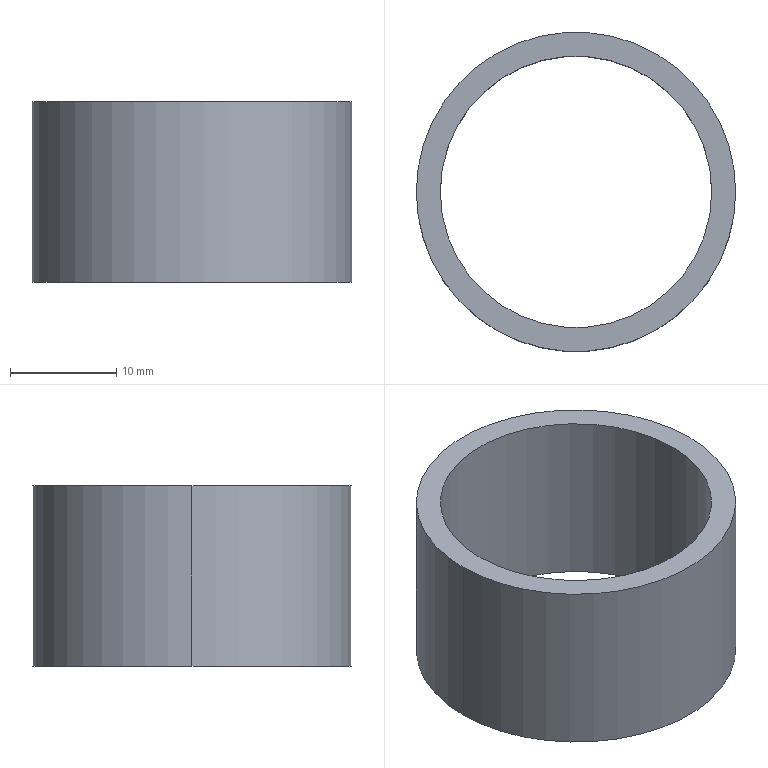Part | SolidWorks | features Extrusion 1 | 1 solid | 6 faces | box 30 x 30 x 17 mm | volume 3335 mm3 | cylinder 4 | plane 2 | commonest cylinder face diameters 25.5 x2 30 x2
STEP:
#1=CARTESIAN_POINT('',(-12.75,0.,17.));
#2=VERTEX_POINT('',#1);
#3=CARTESIAN_POINT('',(12.75,0.,17.));
#4=VERTEX_POINT('',#3);
#5=CARTESIAN_POINT('',(0.,0.,17.));
#6=DIRECTION('',(0.,0.,1.));
#7=DIRECTION('',(1.,0.,0.));
#8=AXIS2_PLACEMENT_3D('',#5,#6,#7);
#9=CIRCLE('',#8,12.75);
#10=EDGE_CURVE('',#2,#4,#9,.T.);
#11=ORIENTED_EDGE('',*,*,#10,.T.);
#12=CARTESIAN_POINT('',(12.75,0.,0.));
#13=VERTEX_POINT('',#12);
#14=CARTESIAN_POINT('',(12.75,0.,17.));
#15=DIRECTION('',(0.,0.,-1.));
#16=VECTOR('',#15,1000.);
#17=LINE('',#14,#16);
#18=EDGE_CURVE('',#4,#13,#17,.T.);
#19=ORIENTED_EDGE('',*,*,#18,.T.);
#20=CARTESIAN_POINT('',(-12.75,0.,0.));
#21=VERTEX_POINT('',#20);
#22=CARTESIAN_POINT('',(0.,0.,0.));
#23=DIRECTION('',(0.,0.,1.));
#24=DIRECTION('',(1.,0.,0.));
#25=AXIS2_PLACEMENT_3D('',#22,#23,#24);
#26=CIRCLE('',#25,12.75);
#27=EDGE_CURVE('',#21,#13,#26,.T.);
#28=ORIENTED_EDGE('',*,*,#27,.F.);
#29=CARTESIAN_POINT('',(-12.75,0.,17.));
#30=DIRECTION('',(0.,0.,-1.));
#31=VECTOR('',#30,1000.);
#32=LINE('',#29,#31);
#33=EDGE_CURVE('',#2,#21,#32,.T.);
#34=ORIENTED_EDGE('',*,*,#33,.F.);
#35=EDGE_LOOP('',(#11,#19,#28,#34));
#36=FACE_OUTER_BOUND('',#35,.T.);
#37=CARTESIAN_POINT('',(0.,0.,17.));
#38=DIRECTION('',(0.,0.,-1.));
#39=DIRECTION('',(-1.,0.,0.));
#40=AXIS2_PLACEMENT_3D('',#37,#38,#39);
#41=CYLINDRICAL_SURFACE('',#40,12.75);
#42=ADVANCED_FACE('',(#36),#41,.F.);
#43=CARTESIAN_POINT('',(15.,0.,17.));
#44=VERTEX_POINT('',#43);
#45=CARTESIAN_POINT('',(-15.,0.,17.));
#46=VERTEX_POINT('',#45);
#47=CARTESIAN_POINT('',(0.,0.,17.));
#48=DIRECTION('',(0.,0.,1.));
#49=DIRECTION('',(1.,0.,0.));
#50=AXIS2_PLACEMENT_3D('',#47,#48,#49);
#51=CIRCLE('',#50,15.);
#52=EDGE_CURVE('',#44,#46,#51,.T.);
#53=ORIENTED_EDGE('',*,*,#52,.F.);
#54=CARTESIAN_POINT('',(15.,0.,0.));
#55=VERTEX_POINT('',#54);
#56=CARTESIAN_POINT('',(15.,0.,17.));
#57=DIRECTION('',(0.,0.,-1.));
#58=VECTOR('',#57,1000.);
#59=LINE('',#56,#58);
#60=EDGE_CURVE('',#44,#55,#59,.T.);
#61=ORIENTED_EDGE('',*,*,#60,.T.);
#62=CARTESIAN_POINT('',(-15.,0.,0.));
#63=VERTEX_POINT('',#62);
#64=CARTESIAN_POINT('',(0.,0.,0.));
#65=DIRECTION('',(0.,0.,1.));
#66=DIRECTION('',(1.,0.,0.));
#67=AXIS2_PLACEMENT_3D('',#64,#65,#66);
#68=CIRCLE('',#67,15.);
#69=EDGE_CURVE('',#55,#63,#68,.T.);
#70=ORIENTED_EDGE('',*,*,#69,.T.);
#71=CARTESIAN_POINT('',(-15.,0.,17.));
#72=DIRECTION('',(0.,0.,-1.));
#73=VECTOR('',#72,1000.);
#74=LINE('',#71,#73);
#75=EDGE_CURVE('',#46,#63,#74,.T.);
#76=ORIENTED_EDGE('',*,*,#75,.F.);
#77=EDGE_LOOP('',(#53,#61,#70,#76));
#78=FACE_OUTER_BOUND('',#77,.T.);
#79=CARTESIAN_POINT('',(0.,0.,17.));
#80=DIRECTION('',(0.,0.,-1.));
#81=DIRECTION('',(-1.,0.,0.));
#82=AXIS2_PLACEMENT_3D('',#79,#80,#81);
#83=CYLINDRICAL_SURFACE('',#82,15.);
#84=ADVANCED_FACE('',(#78),#83,.T.);
#85=CARTESIAN_POINT('',(0.,0.,17.));
#86=DIRECTION('',(0.,0.,1.));
#87=DIRECTION('',(1.,0.,0.));
#88=AXIS2_PLACEMENT_3D('',#85,#86,#87);
#89=CIRCLE('',#88,15.);
#90=EDGE_CURVE('',#46,#44,#89,.T.);
#91=ORIENTED_EDGE('',*,*,#90,.T.);
#92=ORIENTED_EDGE('',*,*,#52,.T.);
#93=EDGE_LOOP('',(#91,#92));
#94=FACE_OUTER_BOUND('',#93,.T.);
#95=ORIENTED_EDGE('',*,*,#10,.F.);
#96=CARTESIAN_POINT('',(0.,0.,17.));
#97=DIRECTION('',(0.,0.,1.));
#98=DIRECTION('',(1.,0.,0.));
#99=AXIS2_PLACEMENT_3D('',#96,#97,#98);
#100=CIRCLE('',#99,12.75);
#101=EDGE_CURVE('',#4,#2,#100,.T.);
#102=ORIENTED_EDGE('',*,*,#101,.F.);
#103=EDGE_LOOP('',(#95,#102));
#104=FACE_BOUND('',#103,.T.);
#105=CARTESIAN_POINT('',(0.,0.,17.));
#106=DIRECTION('',(0.,0.,1.));
#107=DIRECTION('',(1.,0.,0.));
#108=AXIS2_PLACEMENT_3D('',#105,#106,#107);
#109=PLANE('',#108);
#110=ADVANCED_FACE('',(#94,#104),#109,.T.);
#111=CARTESIAN_POINT('',(0.,0.,0.));
#112=DIRECTION('',(0.,0.,1.));
#113=DIRECTION('',(1.,0.,0.));
#114=AXIS2_PLACEMENT_3D('',#111,#112,#113);
#115=CIRCLE('',#114,15.);
#116=EDGE_CURVE('',#63,#55,#115,.T.);
#117=ORIENTED_EDGE('',*,*,#116,.F.);
#118=ORIENTED_EDGE('',*,*,#69,.F.);
#119=EDGE_LOOP('',(#117,#118));
#120=FACE_OUTER_BOUND('',#119,.T.);
#121=ORIENTED_EDGE('',*,*,#27,.T.);
#122=CARTESIAN_POINT('',(0.,0.,0.));
#123=DIRECTION('',(0.,0.,1.));
#124=DIRECTION('',(1.,0.,0.));
#125=AXIS2_PLACEMENT_3D('',#122,#123,#124);
#126=CIRCLE('',#125,12.75);
#127=EDGE_CURVE('',#13,#21,#126,.T.);
#128=ORIENTED_EDGE('',*,*,#127,.T.);
#129=EDGE_LOOP('',(#121,#128));
#130=FACE_BOUND('',#129,.T.);
#131=CARTESIAN_POINT('',(0.,0.,0.));
#132=DIRECTION('',(0.,0.,1.));
#133=DIRECTION('',(1.,0.,0.));
#134=AXIS2_PLACEMENT_3D('',#131,#132,#133);
#135=PLANE('',#134);
#136=ADVANCED_FACE('',(#120,#130),#135,.F.);
#137=ORIENTED_EDGE('',*,*,#60,.F.);
#138=ORIENTED_EDGE('',*,*,#90,.F.);
#139=ORIENTED_EDGE('',*,*,#75,.T.);
#140=ORIENTED_EDGE('',*,*,#116,.T.);
#141=EDGE_LOOP('',(#137,#138,#139,#140));
#142=FACE_OUTER_BOUND('',#141,.T.);
#143=CARTESIAN_POINT('',(0.,0.,17.));
#144=DIRECTION('',(0.,0.,-1.));
#145=DIRECTION('',(-1.,0.,0.));
#146=AXIS2_PLACEMENT_3D('',#143,#144,#145);
#147=CYLINDRICAL_SURFACE('',#146,15.);
#148=ADVANCED_FACE('',(#142),#147,.T.);
#149=ORIENTED_EDGE('',*,*,#18,.F.);
#150=ORIENTED_EDGE('',*,*,#101,.T.);
#151=ORIENTED_EDGE('',*,*,#33,.T.);
#152=ORIENTED_EDGE('',*,*,#127,.F.);
#153=EDGE_LOOP('',(#149,#150,#151,#152));
#154=FACE_OUTER_BOUND('',#153,.T.);
#155=CARTESIAN_POINT('',(0.,0.,17.));
#156=DIRECTION('',(0.,0.,-1.));
#157=DIRECTION('',(-1.,0.,0.));
#158=AXIS2_PLACEMENT_3D('',#155,#156,#157);
#159=CYLINDRICAL_SURFACE('',#158,12.75);
#160=ADVANCED_FACE('',(#154),#159,.F.);
#161=CLOSED_SHELL('',(#42,#84,#110,#136,#148,#160));
#162=MANIFOLD_SOLID_BREP('',#161);
#163=CARTESIAN_POINT('',(0.,0.,0.));
#164=DIRECTION('',(0.,0.,1.));
#165=DIRECTION('',(1.,0.,0.));
#166=AXIS2_PLACEMENT_3D('',#163,#164,#165);
#167=(LENGTH_UNIT()NAMED_UNIT(*)SI_UNIT(.MILLI.,.METRE.));
#168=UNCERTAINTY_MEASURE_WITH_UNIT(LENGTH_MEASURE(0.00001),#167,'','');
#169=(NAMED_UNIT(*)PLANE_ANGLE_UNIT()SI_UNIT($,.RADIAN.));
#170=(NAMED_UNIT(*)SI_UNIT($,.STERADIAN.)SOLID_ANGLE_UNIT());
#171=(GEOMETRIC_REPRESENTATION_CONTEXT(3)GLOBAL_UNCERTAINTY_ASSIGNED_CONTEXT((#168))GLOBAL_UNIT_ASSIGNED_CONTEXT((#167,#169,#170))REPRESENTATION_CONTEXT('',''));
#172=ADVANCED_BREP_SHAPE_REPRESENTATION('',(#162,#166),#171);